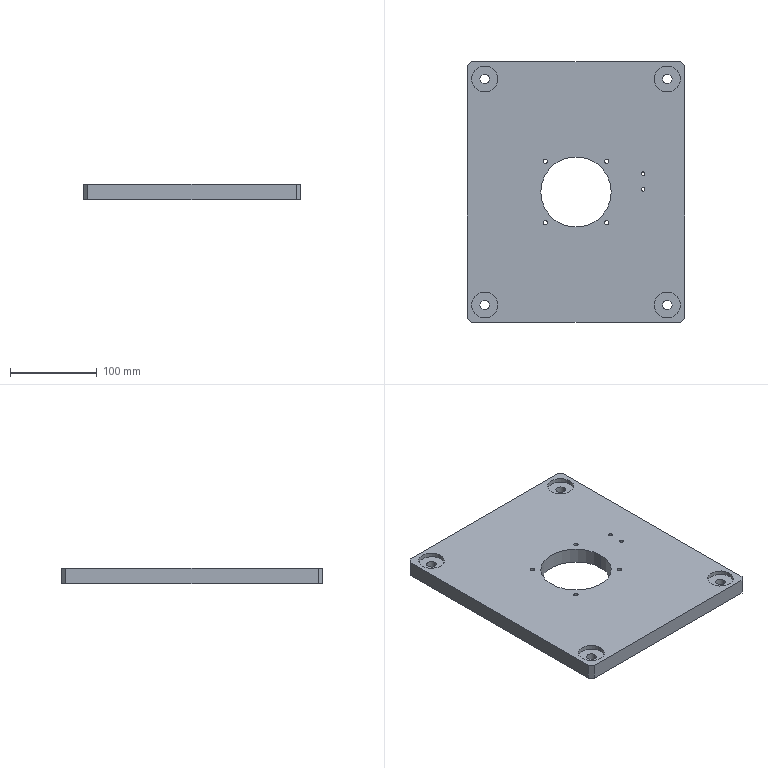Part | STEP file | BB013A02M-04-08A | 1 solid | 44 faces | box 250 x 300 x 18 mm | volume 1235355 mm3 | cylinder 30 | plane 14 | commonest cylinder face diameters 5 x8 11 x8 30 x8 4.2 x4 81 x2